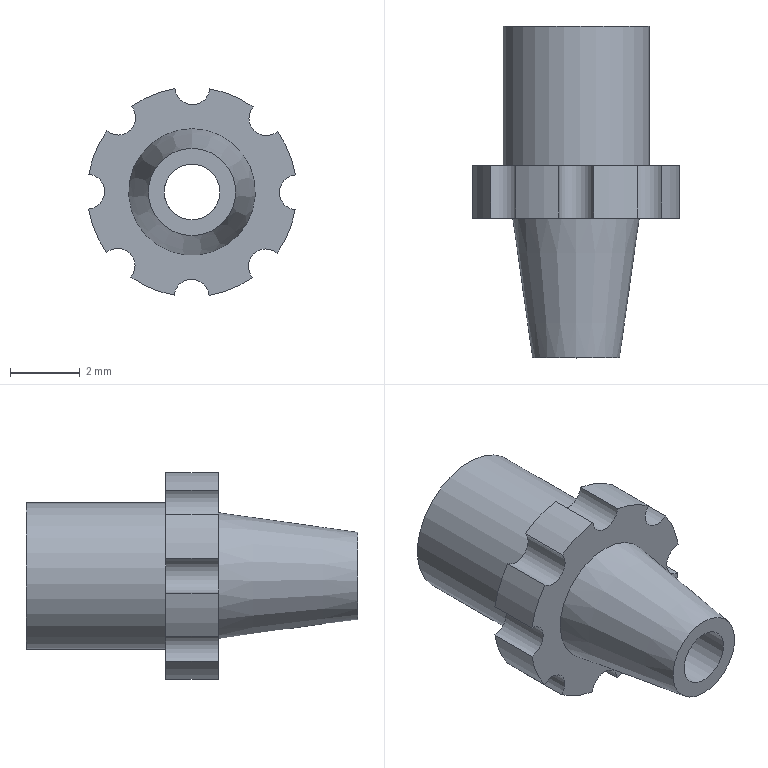Part | NX | features EXTRUDE 12, EXTRACT_STRING 8, Instance Feature 7, DATUM_CSYS 5, SKETCH 4, DRAFT 1, Pattern Feature 1, SYMBOLIC_THREAD 1 | 1 solid | 23 faces | box 5.92 x 9.5 x 5.92 mm | volume 103.972 mm3 | cylinder 18 | plane 4 | cone 1 | commonest cylinder face diameters 1 x8 6 x8 1.6 x1 4.2 x1
STEP:
#1=CARTESIAN_POINT('',(2.451,0.,1.73));
#2=VERTEX_POINT('',#1);
#3=CARTESIAN_POINT('',(2.96,0.,0.4868));
#4=VERTEX_POINT('',#3);
#5=CARTESIAN_POINT('',(0.,0.,0.));
#6=DIRECTION('',(0.,1.,0.));
#7=DIRECTION('',(1.,0.,0.));
#8=AXIS2_PLACEMENT_3D('',#5,#6,#7);
#9=CIRCLE('',#8,3.);
#10=EDGE_CURVE('',#2,#4,#9,.T.);
#11=ORIENTED_EDGE('',*,*,#10,.F.);
#12=CARTESIAN_POINT('',(2.451,-1.5,1.73));
#13=VERTEX_POINT('',#12);
#14=CARTESIAN_POINT('',(2.451,-0.75,1.73));
#15=DIRECTION('',(0.,1.,0.));
#16=VECTOR('',#15,1000.);
#17=LINE('',#14,#16);
#18=EDGE_CURVE('',#2,#13,#17,.F.);
#19=ORIENTED_EDGE('',*,*,#18,.T.);
#20=CARTESIAN_POINT('',(2.96,-1.5,0.4868));
#21=VERTEX_POINT('',#20);
#22=CARTESIAN_POINT('',(0.,-1.5,0.));
#23=DIRECTION('',(0.,1.,0.));
#24=DIRECTION('',(1.,0.,0.));
#25=AXIS2_PLACEMENT_3D('',#22,#23,#24);
#26=CIRCLE('',#25,3.);
#27=EDGE_CURVE('',#13,#21,#26,.T.);
#28=ORIENTED_EDGE('',*,*,#27,.T.);
#29=CARTESIAN_POINT('',(2.96,-0.75,0.4868));
#30=DIRECTION('',(0.,1.,0.));
#31=VECTOR('',#30,1000.);
#32=LINE('',#29,#31);
#33=EDGE_CURVE('',#21,#4,#32,.T.);
#34=ORIENTED_EDGE('',*,*,#33,.T.);
#35=EDGE_LOOP('',(#11,#19,#28,#34));
#36=FACE_BOUND('',#35,.T.);
#37=CARTESIAN_POINT('',(0.,-1.5,0.));
#38=DIRECTION('',(0.,1.,0.));
#39=DIRECTION('',(0.,0.,1.));
#40=AXIS2_PLACEMENT_3D('',#37,#38,#39);
#41=CYLINDRICAL_SURFACE('',#40,3.);
#42=ADVANCED_FACE('',(#36),#41,.T.);
#43=CARTESIAN_POINT('',(0.5097,-1.5,2.956));
#44=VERTEX_POINT('',#43);
#45=CARTESIAN_POINT('',(1.749,-1.5,2.437));
#46=VERTEX_POINT('',#45);
#47=CARTESIAN_POINT('',(0.,-1.5,0.));
#48=DIRECTION('',(0.,1.,0.));
#49=DIRECTION('',(1.,0.,0.));
#50=AXIS2_PLACEMENT_3D('',#47,#48,#49);
#51=CIRCLE('',#50,3.);
#52=EDGE_CURVE('',#44,#46,#51,.T.);
#53=ORIENTED_EDGE('',*,*,#52,.T.);
#54=CARTESIAN_POINT('',(1.749,0.,2.437));
#55=VERTEX_POINT('',#54);
#56=CARTESIAN_POINT('',(1.749,-0.75,2.437));
#57=DIRECTION('',(0.,1.,0.));
#58=VECTOR('',#57,1000.);
#59=LINE('',#56,#58);
#60=EDGE_CURVE('',#46,#55,#59,.T.);
#61=ORIENTED_EDGE('',*,*,#60,.T.);
#62=CARTESIAN_POINT('',(0.5097,0.,2.956));
#63=VERTEX_POINT('',#62);
#64=CARTESIAN_POINT('',(0.,0.,0.));
#65=DIRECTION('',(0.,1.,0.));
#66=DIRECTION('',(1.,0.,0.));
#67=AXIS2_PLACEMENT_3D('',#64,#65,#66);
#68=CIRCLE('',#67,3.);
#69=EDGE_CURVE('',#63,#55,#68,.T.);
#70=ORIENTED_EDGE('',*,*,#69,.F.);
#71=CARTESIAN_POINT('',(0.5097,-0.75,2.956));
#72=DIRECTION('',(0.,1.,0.));
#73=VECTOR('',#72,1000.);
#74=LINE('',#71,#73);
#75=EDGE_CURVE('',#63,#44,#74,.F.);
#76=ORIENTED_EDGE('',*,*,#75,.T.);
#77=EDGE_LOOP('',(#53,#61,#70,#76));
#78=FACE_BOUND('',#77,.T.);
#79=CARTESIAN_POINT('',(0.,-1.5,0.));
#80=DIRECTION('',(0.,1.,0.));
#81=DIRECTION('',(0.,0.,1.));
#82=AXIS2_PLACEMENT_3D('',#79,#80,#81);
#83=CYLINDRICAL_SURFACE('',#82,3.);
#84=ADVANCED_FACE('',(#78),#83,.T.);
#85=CARTESIAN_POINT('',(2.956,0.,-0.5097));
#86=VERTEX_POINT('',#85);
#87=CARTESIAN_POINT('',(2.437,0.,-1.749));
#88=VERTEX_POINT('',#87);
#89=CARTESIAN_POINT('',(0.,0.,0.));
#90=DIRECTION('',(0.,1.,0.));
#91=DIRECTION('',(1.,0.,0.));
#92=AXIS2_PLACEMENT_3D('',#89,#90,#91);
#93=CIRCLE('',#92,3.);
#94=EDGE_CURVE('',#86,#88,#93,.T.);
#95=ORIENTED_EDGE('',*,*,#94,.F.);
#96=CARTESIAN_POINT('',(2.956,-1.5,-0.5097));
#97=VERTEX_POINT('',#96);
#98=CARTESIAN_POINT('',(2.956,-0.75,-0.5097));
#99=DIRECTION('',(0.,1.,0.));
#100=VECTOR('',#99,1000.);
#101=LINE('',#98,#100);
#102=EDGE_CURVE('',#86,#97,#101,.F.);
#103=ORIENTED_EDGE('',*,*,#102,.T.);
#104=CARTESIAN_POINT('',(2.437,-1.5,-1.749));
#105=VERTEX_POINT('',#104);
#106=CARTESIAN_POINT('',(0.,-1.5,0.));
#107=DIRECTION('',(0.,1.,0.));
#108=DIRECTION('',(1.,0.,0.));
#109=AXIS2_PLACEMENT_3D('',#106,#107,#108);
#110=CIRCLE('',#109,3.);
#111=EDGE_CURVE('',#97,#105,#110,.T.);
#112=ORIENTED_EDGE('',*,*,#111,.T.);
#113=CARTESIAN_POINT('',(2.437,-0.75,-1.749));
#114=DIRECTION('',(0.,1.,0.));
#115=VECTOR('',#114,1000.);
#116=LINE('',#113,#115);
#117=EDGE_CURVE('',#105,#88,#116,.T.);
#118=ORIENTED_EDGE('',*,*,#117,.T.);
#119=EDGE_LOOP('',(#95,#103,#112,#118));
#120=FACE_BOUND('',#119,.T.);
#121=CARTESIAN_POINT('',(0.,-1.5,0.));
#122=DIRECTION('',(0.,1.,0.));
#123=DIRECTION('',(0.,0.,1.));
#124=AXIS2_PLACEMENT_3D('',#121,#122,#123);
#125=CYLINDRICAL_SURFACE('',#124,3.);
#126=ADVANCED_FACE('',(#120),#125,.T.);
#127=CARTESIAN_POINT('',(1.73,0.,-2.451));
#128=VERTEX_POINT('',#127);
#129=CARTESIAN_POINT('',(0.4868,0.,-2.96));
#130=VERTEX_POINT('',#129);
#131=CARTESIAN_POINT('',(0.,0.,0.));
#132=DIRECTION('',(0.,1.,0.));
#133=DIRECTION('',(1.,0.,0.));
#134=AXIS2_PLACEMENT_3D('',#131,#132,#133);
#135=CIRCLE('',#134,3.);
#136=EDGE_CURVE('',#128,#130,#135,.T.);
#137=ORIENTED_EDGE('',*,*,#136,.F.);
#138=CARTESIAN_POINT('',(1.73,-1.5,-2.451));
#139=VERTEX_POINT('',#138);
#140=CARTESIAN_POINT('',(1.73,-0.75,-2.451));
#141=DIRECTION('',(0.,1.,0.));
#142=VECTOR('',#141,1000.);
#143=LINE('',#140,#142);
#144=EDGE_CURVE('',#128,#139,#143,.F.);
#145=ORIENTED_EDGE('',*,*,#144,.T.);
#146=CARTESIAN_POINT('',(0.4868,-1.5,-2.96));
#147=VERTEX_POINT('',#146);
#148=CARTESIAN_POINT('',(0.,-1.5,0.));
#149=DIRECTION('',(0.,1.,0.));
#150=DIRECTION('',(1.,0.,0.));
#151=AXIS2_PLACEMENT_3D('',#148,#149,#150);
#152=CIRCLE('',#151,3.);
#153=EDGE_CURVE('',#139,#147,#152,.T.);
#154=ORIENTED_EDGE('',*,*,#153,.T.);
#155=CARTESIAN_POINT('',(0.4868,-0.75,-2.96));
#156=DIRECTION('',(0.,1.,0.));
#157=VECTOR('',#156,1000.);
#158=LINE('',#155,#157);
#159=EDGE_CURVE('',#147,#130,#158,.T.);
#160=ORIENTED_EDGE('',*,*,#159,.T.);
#161=EDGE_LOOP('',(#137,#145,#154,#160));
#162=FACE_BOUND('',#161,.T.);
#163=CARTESIAN_POINT('',(0.,-1.5,0.));
#164=DIRECTION('',(0.,1.,0.));
#165=DIRECTION('',(0.,0.,1.));
#166=AXIS2_PLACEMENT_3D('',#163,#164,#165);
#167=CYLINDRICAL_SURFACE('',#166,3.);
#168=ADVANCED_FACE('',(#162),#167,.T.);
#169=CARTESIAN_POINT('',(-0.5097,0.,-2.956));
#170=VERTEX_POINT('',#169);
#171=CARTESIAN_POINT('',(-1.749,0.,-2.437));
#172=VERTEX_POINT('',#171);
#173=CARTESIAN_POINT('',(0.,0.,0.));
#174=DIRECTION('',(0.,1.,0.));
#175=DIRECTION('',(1.,0.,0.));
#176=AXIS2_PLACEMENT_3D('',#173,#174,#175);
#177=CIRCLE('',#176,3.);
#178=EDGE_CURVE('',#170,#172,#177,.T.);
#179=ORIENTED_EDGE('',*,*,#178,.F.);
#180=CARTESIAN_POINT('',(-0.5097,-1.5,-2.956));
#181=VERTEX_POINT('',#180);
#182=CARTESIAN_POINT('',(-0.5097,-0.75,-2.956));
#183=DIRECTION('',(0.,1.,0.));
#184=VECTOR('',#183,1000.);
#185=LINE('',#182,#184);
#186=EDGE_CURVE('',#170,#181,#185,.F.);
#187=ORIENTED_EDGE('',*,*,#186,.T.);
#188=CARTESIAN_POINT('',(-1.749,-1.5,-2.437));
#189=VERTEX_POINT('',#188);
#190=CARTESIAN_POINT('',(0.,-1.5,0.));
#191=DIRECTION('',(0.,1.,0.));
#192=DIRECTION('',(1.,0.,0.));
#193=AXIS2_PLACEMENT_3D('',#190,#191,#192);
#194=CIRCLE('',#193,3.);
#195=EDGE_CURVE('',#181,#189,#194,.T.);
#196=ORIENTED_EDGE('',*,*,#195,.T.);
#197=CARTESIAN_POINT('',(-1.749,-0.75,-2.437));
#198=DIRECTION('',(0.,1.,0.));
#199=VECTOR('',#198,1000.);
#200=LINE('',#197,#199);
#201=EDGE_CURVE('',#189,#172,#200,.T.);
#202=ORIENTED_EDGE('',*,*,#201,.T.);
#203=EDGE_LOOP('',(#179,#187,#196,#202));
#204=FACE_BOUND('',#203,.T.);
#205=CARTESIAN_POINT('',(0.,-1.5,0.));
#206=DIRECTION('',(0.,1.,0.));
#207=DIRECTION('',(0.,0.,1.));
#208=AXIS2_PLACEMENT_3D('',#205,#206,#207);
#209=CYLINDRICAL_SURFACE('',#208,3.);
#210=ADVANCED_FACE('',(#204),#209,.T.);
#211=CARTESIAN_POINT('',(-2.451,0.,-1.73));
#212=VERTEX_POINT('',#211);
#213=CARTESIAN_POINT('',(-2.96,0.,-0.4868));
#214=VERTEX_POINT('',#213);
#215=CARTESIAN_POINT('',(0.,0.,0.));
#216=DIRECTION('',(0.,1.,0.));
#217=DIRECTION('',(1.,0.,0.));
#218=AXIS2_PLACEMENT_3D('',#215,#216,#217);
#219=CIRCLE('',#218,3.);
#220=EDGE_CURVE('',#212,#214,#219,.T.);
#221=ORIENTED_EDGE('',*,*,#220,.F.);
#222=CARTESIAN_POINT('',(-2.451,-1.5,-1.73));
#223=VERTEX_POINT('',#222);
#224=CARTESIAN_POINT('',(-2.451,-0.75,-1.73));
#225=DIRECTION('',(0.,1.,0.));
#226=VECTOR('',#225,1000.);
#227=LINE('',#224,#226);
#228=EDGE_CURVE('',#212,#223,#227,.F.);
#229=ORIENTED_EDGE('',*,*,#228,.T.);
#230=CARTESIAN_POINT('',(-2.96,-1.5,-0.4868));
#231=VERTEX_POINT('',#230);
#232=CARTESIAN_POINT('',(0.,-1.5,0.));
#233=DIRECTION('',(0.,1.,0.));
#234=DIRECTION('',(1.,0.,0.));
#235=AXIS2_PLACEMENT_3D('',#232,#233,#234);
#236=CIRCLE('',#235,3.);
#237=EDGE_CURVE('',#223,#231,#236,.T.);
#238=ORIENTED_EDGE('',*,*,#237,.T.);
#239=CARTESIAN_POINT('',(-2.96,-0.75,-0.4868));
#240=DIRECTION('',(0.,1.,0.));
#241=VECTOR('',#240,1000.);
#242=LINE('',#239,#241);
#243=EDGE_CURVE('',#231,#214,#242,.T.);
#244=ORIENTED_EDGE('',*,*,#243,.T.);
#245=EDGE_LOOP('',(#221,#229,#238,#244));
#246=FACE_BOUND('',#245,.T.);
#247=CARTESIAN_POINT('',(0.,-1.5,0.));
#248=DIRECTION('',(0.,1.,0.));
#249=DIRECTION('',(0.,0.,1.));
#250=AXIS2_PLACEMENT_3D('',#247,#248,#249);
#251=CYLINDRICAL_SURFACE('',#250,3.);
#252=ADVANCED_FACE('',(#246),#251,.T.);
#253=CARTESIAN_POINT('',(-2.956,0.,0.5097));
#254=VERTEX_POINT('',#253);
#255=CARTESIAN_POINT('',(-2.437,0.,1.749));
#256=VERTEX_POINT('',#255);
#257=CARTESIAN_POINT('',(0.,0.,0.));
#258=DIRECTION('',(0.,1.,0.));
#259=DIRECTION('',(1.,0.,0.));
#260=AXIS2_PLACEMENT_3D('',#257,#258,#259);
#261=CIRCLE('',#260,3.);
#262=EDGE_CURVE('',#254,#256,#261,.T.);
#263=ORIENTED_EDGE('',*,*,#262,.F.);
#264=CARTESIAN_POINT('',(-2.956,-1.5,0.5097));
#265=VERTEX_POINT('',#264);
#266=CARTESIAN_POINT('',(-2.956,-0.75,0.5097));
#267=DIRECTION('',(0.,1.,0.));
#268=VECTOR('',#267,1000.);
#269=LINE('',#266,#268);
#270=EDGE_CURVE('',#254,#265,#269,.F.);
#271=ORIENTED_EDGE('',*,*,#270,.T.);
#272=CARTESIAN_POINT('',(-2.437,-1.5,1.749));
#273=VERTEX_POINT('',#272);
#274=CARTESIAN_POINT('',(0.,-1.5,0.));
#275=DIRECTION('',(0.,1.,0.));
#276=DIRECTION('',(1.,0.,0.));
#277=AXIS2_PLACEMENT_3D('',#274,#275,#276);
#278=CIRCLE('',#277,3.);
#279=EDGE_CURVE('',#265,#273,#278,.T.);
#280=ORIENTED_EDGE('',*,*,#279,.T.);
#281=CARTESIAN_POINT('',(-2.437,-0.75,1.749));
#282=DIRECTION('',(0.,1.,0.));
#283=VECTOR('',#282,1000.);
#284=LINE('',#281,#283);
#285=EDGE_CURVE('',#273,#256,#284,.T.);
#286=ORIENTED_EDGE('',*,*,#285,.T.);
#287=EDGE_LOOP('',(#263,#271,#280,#286));
#288=FACE_BOUND('',#287,.T.);
#289=CARTESIAN_POINT('',(0.,-1.5,0.));
#290=DIRECTION('',(0.,1.,0.));
#291=DIRECTION('',(0.,0.,1.));
#292=AXIS2_PLACEMENT_3D('',#289,#290,#291);
#293=CYLINDRICAL_SURFACE('',#292,3.);
#294=ADVANCED_FACE('',(#288),#293,.T.);
#295=CARTESIAN_POINT('',(-1.73,0.,2.451));
#296=VERTEX_POINT('',#295);
#297=CARTESIAN_POINT('',(-0.4868,0.,2.96));
#298=VERTEX_POINT('',#297);
#299=CARTESIAN_POINT('',(0.,0.,0.));
#300=DIRECTION('',(0.,1.,0.));
#301=DIRECTION('',(1.,0.,0.));
#302=AXIS2_PLACEMENT_3D('',#299,#300,#301);
#303=CIRCLE('',#302,3.);
#304=EDGE_CURVE('',#296,#298,#303,.T.);
#305=ORIENTED_EDGE('',*,*,#304,.F.);
#306=CARTESIAN_POINT('',(-1.73,-1.5,2.451));
#307=VERTEX_POINT('',#306);
#308=CARTESIAN_POINT('',(-1.73,-0.75,2.451));
#309=DIRECTION('',(0.,1.,0.));
#310=VECTOR('',#309,1000.);
#311=LINE('',#308,#310);
#312=EDGE_CURVE('',#296,#307,#311,.F.);
#313=ORIENTED_EDGE('',*,*,#312,.T.);
#314=CARTESIAN_POINT('',(-0.4868,-1.5,2.96));
#315=VERTEX_POINT('',#314);
#316=CARTESIAN_POINT('',(0.,-1.5,0.));
#317=DIRECTION('',(0.,1.,0.));
#318=DIRECTION('',(1.,0.,0.));
#319=AXIS2_PLACEMENT_3D('',#316,#317,#318);
#320=CIRCLE('',#319,3.);
#321=EDGE_CURVE('',#307,#315,#320,.T.);
#322=ORIENTED_EDGE('',*,*,#321,.T.);
#323=CARTESIAN_POINT('',(-0.4868,-0.75,2.96));
#324=DIRECTION('',(0.,1.,0.));
#325=VECTOR('',#324,1000.);
#326=LINE('',#323,#325);
#327=EDGE_CURVE('',#315,#298,#326,.T.);
#328=ORIENTED_EDGE('',*,*,#327,.T.);
#329=EDGE_LOOP('',(#305,#313,#322,#328));
#330=FACE_BOUND('',#329,.T.);
#331=CARTESIAN_POINT('',(0.,-1.5,0.));
#332=DIRECTION('',(0.,1.,0.));
#333=DIRECTION('',(0.,0.,1.));
#334=AXIS2_PLACEMENT_3D('',#331,#332,#333);
#335=CYLINDRICAL_SURFACE('',#334,3.);
#336=ADVANCED_FACE('',(#330),#335,.T.);
#337=CARTESIAN_POINT('',(2.1,4.,0.));
#338=VERTEX_POINT('',#337);
#339=CARTESIAN_POINT('',(0.,4.,0.));
#340=DIRECTION('',(0.,1.,0.));
#341=DIRECTION('',(1.,0.,0.));
#342=AXIS2_PLACEMENT_3D('',#339,#340,#341);
#343=CIRCLE('',#342,2.1);
#344=EDGE_CURVE('',#338,#338,#343,.T.);
#345=ORIENTED_EDGE('',*,*,#344,.F.);
#346=EDGE_LOOP('',(#345));
#347=FACE_BOUND('',#346,.T.);
#348=CARTESIAN_POINT('',(2.1,0.,0.));
#349=VERTEX_POINT('',#348);
#350=CARTESIAN_POINT('',(0.,0.,0.));
#351=DIRECTION('',(0.,1.,0.));
#352=DIRECTION('',(1.,0.,0.));
#353=AXIS2_PLACEMENT_3D('',#350,#351,#352);
#354=CIRCLE('',#353,2.1);
#355=EDGE_CURVE('',#349,#349,#354,.T.);
#356=ORIENTED_EDGE('',*,*,#355,.T.);
#357=EDGE_LOOP('',(#356));
#358=FACE_BOUND('',#357,.T.);
#359=CARTESIAN_POINT('',(0.,4.,0.));
#360=DIRECTION('',(0.,-1.,0.));
#361=DIRECTION('',(0.,0.,-1.));
#362=AXIS2_PLACEMENT_3D('',#359,#360,#361);
#363=CYLINDRICAL_SURFACE('',#362,2.1);
#364=ADVANCED_FACE('',(#347,#358),#363,.T.);
#365=CARTESIAN_POINT('',(0.,4.,0.8));
#366=VERTEX_POINT('',#365);
#367=CARTESIAN_POINT('',(0.,4.,0.));
#368=DIRECTION('',(0.,1.,0.));
#369=DIRECTION('',(0.,0.,1.));
#370=AXIS2_PLACEMENT_3D('',#367,#368,#369);
#371=CIRCLE('',#370,0.8);
#372=EDGE_CURVE('',#366,#366,#371,.F.);
#373=ORIENTED_EDGE('',*,*,#372,.T.);
#374=EDGE_LOOP('',(#373));
#375=FACE_BOUND('',#374,.T.);
#376=ORIENTED_EDGE('',*,*,#344,.T.);
#377=EDGE_LOOP('',(#376));
#378=FACE_BOUND('',#377,.T.);
#379=CARTESIAN_POINT('',(0.,4.,0.));
#380=DIRECTION('',(0.,1.,0.));
#381=DIRECTION('',(0.,0.,1.));
#382=AXIS2_PLACEMENT_3D('',#379,#380,#381);
#383=PLANE('',#382);
#384=ADVANCED_FACE('',(#375,#378),#383,.T.);
#385=CARTESIAN_POINT('',(0.,-1.5,1.812));
#386=VERTEX_POINT('',#385);
#387=CARTESIAN_POINT('',(0.,-1.5,0.));
#388=DIRECTION('',(0.,1.,0.));
#389=DIRECTION('',(0.,0.,1.));
#390=AXIS2_PLACEMENT_3D('',#387,#388,#389);
#391=CIRCLE('',#390,1.812);
#392=EDGE_CURVE('',#386,#386,#391,.T.);
#393=ORIENTED_EDGE('',*,*,#392,.T.);
#394=EDGE_LOOP('',(#393));
#395=FACE_BOUND('',#394,.T.);
#396=CARTESIAN_POINT('',(2.129,-1.5,2.113));
#397=DIRECTION('',(0.,-1.,0.));
#398=DIRECTION('',(0.7071,0.,-0.7071));
#399=AXIS2_PLACEMENT_3D('',#396,#397,#398);
#400=CIRCLE('',#399,0.5);
#401=EDGE_CURVE('',#46,#13,#400,.T.);
#402=ORIENTED_EDGE('',*,*,#401,.F.);
#403=ORIENTED_EDGE('',*,*,#52,.F.);
#404=CARTESIAN_POINT('',(0.01159,-1.5,3.));
#405=DIRECTION('',(0.,-1.,0.));
#406=DIRECTION('',(1.,0.,0.));
#407=AXIS2_PLACEMENT_3D('',#404,#405,#406);
#408=CIRCLE('',#407,0.5);
#409=EDGE_CURVE('',#315,#44,#408,.T.);
#410=ORIENTED_EDGE('',*,*,#409,.F.);
#411=ORIENTED_EDGE('',*,*,#321,.F.);
#412=CARTESIAN_POINT('',(-2.113,-1.5,2.129));
#413=DIRECTION('',(0.,-1.,0.));
#414=DIRECTION('',(0.7071,0.,0.7071));
#415=AXIS2_PLACEMENT_3D('',#412,#413,#414);
#416=CIRCLE('',#415,0.5);
#417=EDGE_CURVE('',#273,#307,#416,.T.);
#418=ORIENTED_EDGE('',*,*,#417,.F.);
#419=ORIENTED_EDGE('',*,*,#279,.F.);
#420=CARTESIAN_POINT('',(-3.,-1.5,0.01159));
#421=DIRECTION('',(0.,-1.,0.));
#422=DIRECTION('',(0.,0.,1.));
#423=AXIS2_PLACEMENT_3D('',#420,#421,#422);
#424=CIRCLE('',#423,0.5);
#425=EDGE_CURVE('',#231,#265,#424,.T.);
#426=ORIENTED_EDGE('',*,*,#425,.F.);
#427=ORIENTED_EDGE('',*,*,#237,.F.);
#428=CARTESIAN_POINT('',(-2.129,-1.5,-2.113));
#429=DIRECTION('',(0.,-1.,0.));
#430=DIRECTION('',(-0.7071,0.,0.7071));
#431=AXIS2_PLACEMENT_3D('',#428,#429,#430);
#432=CIRCLE('',#431,0.5);
#433=EDGE_CURVE('',#189,#223,#432,.T.);
#434=ORIENTED_EDGE('',*,*,#433,.F.);
#435=ORIENTED_EDGE('',*,*,#195,.F.);
#436=CARTESIAN_POINT('',(-0.01159,-1.5,-3.));
#437=DIRECTION('',(0.,-1.,0.));
#438=DIRECTION('',(-1.,0.,0.));
#439=AXIS2_PLACEMENT_3D('',#436,#437,#438);
#440=CIRCLE('',#439,0.5);
#441=EDGE_CURVE('',#147,#181,#440,.T.);
#442=ORIENTED_EDGE('',*,*,#441,.F.);
#443=ORIENTED_EDGE('',*,*,#153,.F.);
#444=CARTESIAN_POINT('',(2.113,-1.5,-2.129));
#445=DIRECTION('',(0.,-1.,0.));
#446=DIRECTION('',(-0.7071,0.,-0.7071));
#447=AXIS2_PLACEMENT_3D('',#444,#445,#446);
#448=CIRCLE('',#447,0.5);
#449=EDGE_CURVE('',#105,#139,#448,.T.);
#450=ORIENTED_EDGE('',*,*,#449,.F.);
#451=ORIENTED_EDGE('',*,*,#111,.F.);
#452=CARTESIAN_POINT('',(3.,-1.5,-0.01159));
#453=DIRECTION('',(0.,-1.,0.));
#454=DIRECTION('',(0.,0.,-1.));
#455=AXIS2_PLACEMENT_3D('',#452,#453,#454);
#456=CIRCLE('',#455,0.5);
#457=EDGE_CURVE('',#21,#97,#456,.T.);
#458=ORIENTED_EDGE('',*,*,#457,.F.);
#459=ORIENTED_EDGE('',*,*,#27,.F.);
#460=EDGE_LOOP('',(#402,#403,#410,#411,#418,#419,#426,#427,#434,#435,#442,#443,#450,#451,#458,#459));
#461=FACE_BOUND('',#460,.T.);
#462=CARTESIAN_POINT('',(0.,-1.5,0.));
#463=DIRECTION('',(0.,1.,0.));
#464=DIRECTION('',(0.,0.,1.));
#465=AXIS2_PLACEMENT_3D('',#462,#463,#464);
#466=PLANE('',#465);
#467=ADVANCED_FACE('',(#395,#461),#466,.F.);
#468=ORIENTED_EDGE('',*,*,#355,.F.);
#469=EDGE_LOOP('',(#468));
#470=FACE_BOUND('',#469,.T.);
#471=ORIENTED_EDGE('',*,*,#69,.T.);
#472=CARTESIAN_POINT('',(2.129,0.,2.113));
#473=DIRECTION('',(0.,-1.,0.));
#474=DIRECTION('',(0.7071,0.,-0.7071));
#475=AXIS2_PLACEMENT_3D('',#472,#473,#474);
#476=CIRCLE('',#475,0.5);
#477=EDGE_CURVE('',#55,#2,#476,.T.);
#478=ORIENTED_EDGE('',*,*,#477,.T.);
#479=ORIENTED_EDGE('',*,*,#10,.T.);
#480=CARTESIAN_POINT('',(3.,0.,-0.01159));
#481=DIRECTION('',(0.,-1.,0.));
#482=DIRECTION('',(0.,0.,-1.));
#483=AXIS2_PLACEMENT_3D('',#480,#481,#482);
#484=CIRCLE('',#483,0.5);
#485=EDGE_CURVE('',#4,#86,#484,.T.);
#486=ORIENTED_EDGE('',*,*,#485,.T.);
#487=ORIENTED_EDGE('',*,*,#94,.T.);
#488=CARTESIAN_POINT('',(2.113,0.,-2.129));
#489=DIRECTION('',(0.,-1.,0.));
#490=DIRECTION('',(-0.7071,0.,-0.7071));
#491=AXIS2_PLACEMENT_3D('',#488,#489,#490);
#492=CIRCLE('',#491,0.5);
#493=EDGE_CURVE('',#88,#128,#492,.T.);
#494=ORIENTED_EDGE('',*,*,#493,.T.);
#495=ORIENTED_EDGE('',*,*,#136,.T.);
#496=CARTESIAN_POINT('',(-0.01159,0.,-3.));
#497=DIRECTION('',(0.,-1.,0.));
#498=DIRECTION('',(-1.,0.,0.));
#499=AXIS2_PLACEMENT_3D('',#496,#497,#498);
#500=CIRCLE('',#499,0.5);
#501=EDGE_CURVE('',#130,#170,#500,.T.);
#502=ORIENTED_EDGE('',*,*,#501,.T.);
#503=ORIENTED_EDGE('',*,*,#178,.T.);
#504=CARTESIAN_POINT('',(-2.129,0.,-2.113));
#505=DIRECTION('',(0.,-1.,0.));
#506=DIRECTION('',(-0.7071,0.,0.7071));
#507=AXIS2_PLACEMENT_3D('',#504,#505,#506);
#508=CIRCLE('',#507,0.5);
#509=EDGE_CURVE('',#172,#212,#508,.T.);
#510=ORIENTED_EDGE('',*,*,#509,.T.);
#511=ORIENTED_EDGE('',*,*,#220,.T.);
#512=CARTESIAN_POINT('',(-3.,0.,0.01159));
#513=DIRECTION('',(0.,-1.,0.));
#514=DIRECTION('',(0.,0.,1.));
#515=AXIS2_PLACEMENT_3D('',#512,#513,#514);
#516=CIRCLE('',#515,0.5);
#517=EDGE_CURVE('',#214,#254,#516,.T.);
#518=ORIENTED_EDGE('',*,*,#517,.T.);
#519=ORIENTED_EDGE('',*,*,#262,.T.);
#520=CARTESIAN_POINT('',(-2.113,0.,2.129));
#521=DIRECTION('',(0.,-1.,0.));
#522=DIRECTION('',(0.7071,0.,0.7071));
#523=AXIS2_PLACEMENT_3D('',#520,#521,#522);
#524=CIRCLE('',#523,0.5);
#525=EDGE_CURVE('',#256,#296,#524,.T.);
#526=ORIENTED_EDGE('',*,*,#525,.T.);
#527=ORIENTED_EDGE('',*,*,#304,.T.);
#528=CARTESIAN_POINT('',(0.01159,0.,3.));
#529=DIRECTION('',(0.,-1.,0.));
#530=DIRECTION('',(1.,0.,0.));
#531=AXIS2_PLACEMENT_3D('',#528,#529,#530);
#532=CIRCLE('',#531,0.5);
#533=EDGE_CURVE('',#298,#63,#532,.T.);
#534=ORIENTED_EDGE('',*,*,#533,.T.);
#535=EDGE_LOOP('',(#471,#478,#479,#486,#487,#494,#495,#502,#503,#510,#511,#518,#519,#526,#527,#534));
#536=FACE_BOUND('',#535,.T.);
#537=CARTESIAN_POINT('',(0.,0.,0.));
#538=DIRECTION('',(0.,1.,0.));
#539=DIRECTION('',(0.,0.,1.));
#540=AXIS2_PLACEMENT_3D('',#537,#538,#539);
#541=PLANE('',#540);
#542=ADVANCED_FACE('',(#470,#536),#541,.T.);
#543=ORIENTED_EDGE('',*,*,#533,.F.);
#544=ORIENTED_EDGE('',*,*,#327,.F.);
#545=ORIENTED_EDGE('',*,*,#409,.T.);
#546=ORIENTED_EDGE('',*,*,#75,.F.);
#547=EDGE_LOOP('',(#543,#544,#545,#546));
#548=FACE_BOUND('',#547,.T.);
#549=CARTESIAN_POINT('',(0.01159,-1.5,3.));
#550=DIRECTION('',(0.,1.,0.));
#551=DIRECTION('',(0.,0.,1.));
#552=AXIS2_PLACEMENT_3D('',#549,#550,#551);
#553=CYLINDRICAL_SURFACE('',#552,0.5);
#554=ADVANCED_FACE('',(#548),#553,.F.);
#555=ORIENTED_EDGE('',*,*,#525,.F.);
#556=ORIENTED_EDGE('',*,*,#285,.F.);
#557=ORIENTED_EDGE('',*,*,#417,.T.);
#558=ORIENTED_EDGE('',*,*,#312,.F.);
#559=EDGE_LOOP('',(#555,#556,#557,#558));
#560=FACE_BOUND('',#559,.T.);
#561=CARTESIAN_POINT('',(-2.113,-1.5,2.129));
#562=DIRECTION('',(0.,1.,0.));
#563=DIRECTION('',(0.,0.,1.));
#564=AXIS2_PLACEMENT_3D('',#561,#562,#563);
#565=CYLINDRICAL_SURFACE('',#564,0.5);
#566=ADVANCED_FACE('',(#560),#565,.F.);
#567=ORIENTED_EDGE('',*,*,#517,.F.);
#568=ORIENTED_EDGE('',*,*,#243,.F.);
#569=ORIENTED_EDGE('',*,*,#425,.T.);
#570=ORIENTED_EDGE('',*,*,#270,.F.);
#571=EDGE_LOOP('',(#567,#568,#569,#570));
#572=FACE_BOUND('',#571,.T.);
#573=CARTESIAN_POINT('',(-3.,-1.5,0.01159));
#574=DIRECTION('',(0.,1.,0.));
#575=DIRECTION('',(0.,0.,1.));
#576=AXIS2_PLACEMENT_3D('',#573,#574,#575);
#577=CYLINDRICAL_SURFACE('',#576,0.5);
#578=ADVANCED_FACE('',(#572),#577,.F.);
#579=ORIENTED_EDGE('',*,*,#509,.F.);
#580=ORIENTED_EDGE('',*,*,#201,.F.);
#581=ORIENTED_EDGE('',*,*,#433,.T.);
#582=ORIENTED_EDGE('',*,*,#228,.F.);
#583=EDGE_LOOP('',(#579,#580,#581,#582));
#584=FACE_BOUND('',#583,.T.);
#585=CARTESIAN_POINT('',(-2.129,-1.5,-2.113));
#586=DIRECTION('',(0.,1.,0.));
#587=DIRECTION('',(0.,0.,1.));
#588=AXIS2_PLACEMENT_3D('',#585,#586,#587);
#589=CYLINDRICAL_SURFACE('',#588,0.5);
#590=ADVANCED_FACE('',(#584),#589,.F.);
#591=ORIENTED_EDGE('',*,*,#501,.F.);
#592=ORIENTED_EDGE('',*,*,#159,.F.);
#593=ORIENTED_EDGE('',*,*,#441,.T.);
#594=ORIENTED_EDGE('',*,*,#186,.F.);
#595=EDGE_LOOP('',(#591,#592,#593,#594));
#596=FACE_BOUND('',#595,.T.);
#597=CARTESIAN_POINT('',(-0.01159,-1.5,-3.));
#598=DIRECTION('',(0.,1.,0.));
#599=DIRECTION('',(0.,0.,1.));
#600=AXIS2_PLACEMENT_3D('',#597,#598,#599);
#601=CYLINDRICAL_SURFACE('',#600,0.5);
#602=ADVANCED_FACE('',(#596),#601,.F.);
#603=ORIENTED_EDGE('',*,*,#493,.F.);
#604=ORIENTED_EDGE('',*,*,#117,.F.);
#605=ORIENTED_EDGE('',*,*,#449,.T.);
#606=ORIENTED_EDGE('',*,*,#144,.F.);
#607=EDGE_LOOP('',(#603,#604,#605,#606));
#608=FACE_BOUND('',#607,.T.);
#609=CARTESIAN_POINT('',(2.113,-1.5,-2.129));
#610=DIRECTION('',(0.,1.,0.));
#611=DIRECTION('',(0.,0.,1.));
#612=AXIS2_PLACEMENT_3D('',#609,#610,#611);
#613=CYLINDRICAL_SURFACE('',#612,0.5);
#614=ADVANCED_FACE('',(#608),#613,.F.);
#615=ORIENTED_EDGE('',*,*,#485,.F.);
#616=ORIENTED_EDGE('',*,*,#33,.F.);
#617=ORIENTED_EDGE('',*,*,#457,.T.);
#618=ORIENTED_EDGE('',*,*,#102,.F.);
#619=EDGE_LOOP('',(#615,#616,#617,#618));
#620=FACE_BOUND('',#619,.T.);
#621=CARTESIAN_POINT('',(3.,-1.5,-0.01159));
#622=DIRECTION('',(0.,1.,0.));
#623=DIRECTION('',(0.,0.,1.));
#624=AXIS2_PLACEMENT_3D('',#621,#622,#623);
#625=CYLINDRICAL_SURFACE('',#624,0.5);
#626=ADVANCED_FACE('',(#620),#625,.F.);
#627=ORIENTED_EDGE('',*,*,#477,.F.);
#628=ORIENTED_EDGE('',*,*,#60,.F.);
#629=ORIENTED_EDGE('',*,*,#401,.T.);
#630=ORIENTED_EDGE('',*,*,#18,.F.);
#631=EDGE_LOOP('',(#627,#628,#629,#630));
#632=FACE_BOUND('',#631,.T.);
#633=CARTESIAN_POINT('',(2.129,-1.5,2.113));
#634=DIRECTION('',(0.,1.,0.));
#635=DIRECTION('',(0.,0.,1.));
#636=AXIS2_PLACEMENT_3D('',#633,#634,#635);
#637=CYLINDRICAL_SURFACE('',#636,0.5);
#638=ADVANCED_FACE('',(#632),#637,.F.);
#639=CARTESIAN_POINT('',(0.,-5.5,1.25));
#640=VERTEX_POINT('',#639);
#641=CARTESIAN_POINT('',(0.,-5.5,0.));
#642=DIRECTION('',(0.,1.,0.));
#643=DIRECTION('',(0.,0.,1.));
#644=AXIS2_PLACEMENT_3D('',#641,#642,#643);
#645=CIRCLE('',#644,1.25);
#646=EDGE_CURVE('',#640,#640,#645,.T.);
#647=ORIENTED_EDGE('',*,*,#646,.T.);
#648=EDGE_LOOP('',(#647));
#649=FACE_BOUND('',#648,.T.);
#650=ORIENTED_EDGE('',*,*,#392,.F.);
#651=EDGE_LOOP('',(#650));
#652=FACE_BOUND('',#651,.T.);
#653=CARTESIAN_POINT('',(0.,-5.5,0.));
#654=DIRECTION('',(0.,1.,0.));
#655=DIRECTION('',(0.,0.,-1.));
#656=AXIS2_PLACEMENT_3D('',#653,#654,#655);
#657=CONICAL_SURFACE('',#656,1.25,0.1396);
#658=ADVANCED_FACE('',(#649,#652),#657,.T.);
#659=CARTESIAN_POINT('',(0.8,-5.5,0.));
#660=VERTEX_POINT('',#659);
#661=CARTESIAN_POINT('',(0.,-5.5,0.));
#662=DIRECTION('',(0.,1.,0.));
#663=DIRECTION('',(1.,0.,0.));
#664=AXIS2_PLACEMENT_3D('',#661,#662,#663);
#665=CIRCLE('',#664,0.8);
#666=EDGE_CURVE('',#660,#660,#665,.T.);
#667=ORIENTED_EDGE('',*,*,#666,.T.);
#668=EDGE_LOOP('',(#667));
#669=FACE_BOUND('',#668,.T.);
#670=ORIENTED_EDGE('',*,*,#646,.F.);
#671=EDGE_LOOP('',(#670));
#672=FACE_BOUND('',#671,.T.);
#673=CARTESIAN_POINT('',(0.,-5.5,0.));
#674=DIRECTION('',(0.,1.,0.));
#675=DIRECTION('',(0.,0.,1.));
#676=AXIS2_PLACEMENT_3D('',#673,#674,#675);
#677=PLANE('',#676);
#678=ADVANCED_FACE('',(#669,#672),#677,.F.);
#679=ORIENTED_EDGE('',*,*,#372,.F.);
#680=EDGE_LOOP('',(#679));
#681=FACE_BOUND('',#680,.T.);
#682=ORIENTED_EDGE('',*,*,#666,.F.);
#683=EDGE_LOOP('',(#682));
#684=FACE_BOUND('',#683,.T.);
#685=CARTESIAN_POINT('',(0.,94.5,0.));
#686=DIRECTION('',(0.,-1.,0.));
#687=DIRECTION('',(0.,0.,-1.));
#688=AXIS2_PLACEMENT_3D('',#685,#686,#687);
#689=CYLINDRICAL_SURFACE('',#688,0.8);
#690=ADVANCED_FACE('',(#681,#684),#689,.F.);
#691=CLOSED_SHELL('',(#42,#84,#126,#168,#210,#252,#294,#336,#364,#384,#467,#542,#554,#566,#578,#590,#602,#614,#626,#638,#658,#678,#690));
#692=MANIFOLD_SOLID_BREP('',#691);
#693=(LENGTH_UNIT()NAMED_UNIT(*)SI_UNIT(.MILLI.,.METRE.));
#694=UNCERTAINTY_MEASURE_WITH_UNIT(LENGTH_MEASURE(0.00001),#693,'','');
#695=(NAMED_UNIT(*)PLANE_ANGLE_UNIT()SI_UNIT($,.RADIAN.));
#696=(NAMED_UNIT(*)SI_UNIT($,.STERADIAN.)SOLID_ANGLE_UNIT());
#697=(GEOMETRIC_REPRESENTATION_CONTEXT(3)GLOBAL_UNCERTAINTY_ASSIGNED_CONTEXT((#694))GLOBAL_UNIT_ASSIGNED_CONTEXT((#693,#695,#696))REPRESENTATION_CONTEXT('',''));
#698=ADVANCED_BREP_SHAPE_REPRESENTATION('',(#692),#697);